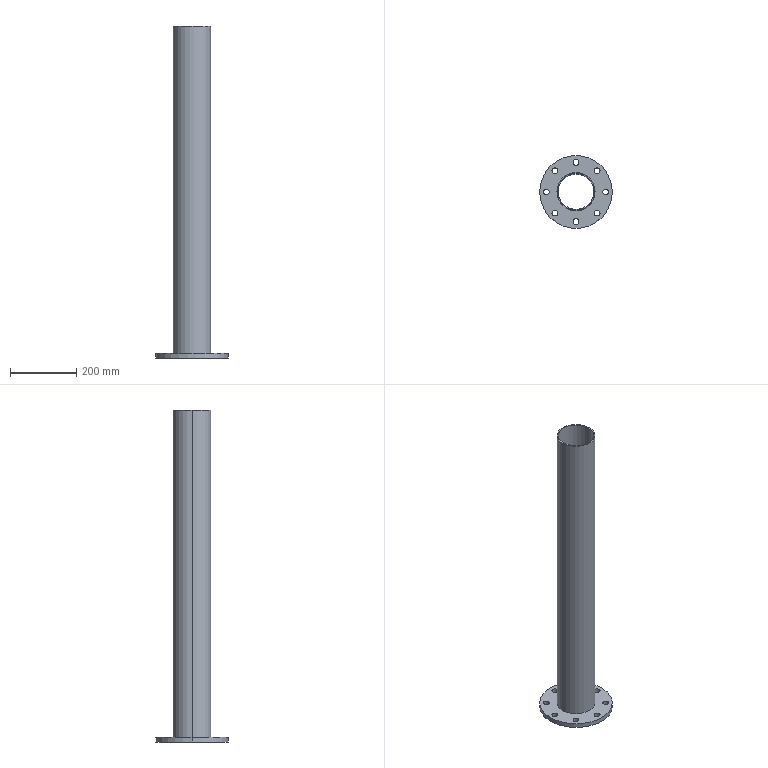Part | SolidWorks | features Extrusion 1, ICE 1 | 2 solids | 28 faces | box 220 x 220 x 1004 mm | volume 1407247 mm3 | cylinder 24 | plane 4 | commonest cylinder face diameters 18 x16 108.3 x2 114.3 x2 115 x2 220 x2
STEP:
#1=CARTESIAN_POINT('',(-72.64,63.64,14.));
#2=VERTEX_POINT('',#1);
#3=CARTESIAN_POINT('',(-54.64,63.64,14.));
#4=VERTEX_POINT('',#3);
#5=CARTESIAN_POINT('',(-63.64,63.64,14.));
#6=DIRECTION('',(0.,0.,1.));
#7=DIRECTION('',(1.,0.,0.));
#8=AXIS2_PLACEMENT_3D('',#5,#6,#7);
#9=CIRCLE('',#8,9.);
#10=EDGE_CURVE('',#2,#4,#9,.T.);
#11=ORIENTED_EDGE('',*,*,#10,.T.);
#12=CARTESIAN_POINT('',(-54.64,63.64,0.));
#13=VERTEX_POINT('',#12);
#14=CARTESIAN_POINT('',(-54.64,63.64,14.));
#15=DIRECTION('',(0.,0.,-1.));
#16=VECTOR('',#15,1000.);
#17=LINE('',#14,#16);
#18=EDGE_CURVE('',#4,#13,#17,.T.);
#19=ORIENTED_EDGE('',*,*,#18,.T.);
#20=CARTESIAN_POINT('',(-72.64,63.64,0.));
#21=VERTEX_POINT('',#20);
#22=CARTESIAN_POINT('',(-63.64,63.64,0.));
#23=DIRECTION('',(0.,0.,1.));
#24=DIRECTION('',(1.,0.,0.));
#25=AXIS2_PLACEMENT_3D('',#22,#23,#24);
#26=CIRCLE('',#25,9.);
#27=EDGE_CURVE('',#21,#13,#26,.T.);
#28=ORIENTED_EDGE('',*,*,#27,.F.);
#29=CARTESIAN_POINT('',(-72.64,63.64,14.));
#30=DIRECTION('',(0.,0.,-1.));
#31=VECTOR('',#30,1000.);
#32=LINE('',#29,#31);
#33=EDGE_CURVE('',#2,#21,#32,.T.);
#34=ORIENTED_EDGE('',*,*,#33,.F.);
#35=EDGE_LOOP('',(#11,#19,#28,#34));
#36=FACE_OUTER_BOUND('',#35,.T.);
#37=CARTESIAN_POINT('',(-63.64,63.64,14.));
#38=DIRECTION('',(0.,0.,-1.));
#39=DIRECTION('',(-1.,0.,0.));
#40=AXIS2_PLACEMENT_3D('',#37,#38,#39);
#41=CYLINDRICAL_SURFACE('',#40,9.);
#42=ADVANCED_FACE('',(#36),#41,.F.);
#43=CARTESIAN_POINT('',(-99.,0.,14.));
#44=VERTEX_POINT('',#43);
#45=CARTESIAN_POINT('',(-81.,0.,14.));
#46=VERTEX_POINT('',#45);
#47=CARTESIAN_POINT('',(-90.,0.,14.));
#48=DIRECTION('',(0.,0.,1.));
#49=DIRECTION('',(1.,0.,0.));
#50=AXIS2_PLACEMENT_3D('',#47,#48,#49);
#51=CIRCLE('',#50,9.);
#52=EDGE_CURVE('',#44,#46,#51,.T.);
#53=ORIENTED_EDGE('',*,*,#52,.T.);
#54=CARTESIAN_POINT('',(-81.,0.,0.));
#55=VERTEX_POINT('',#54);
#56=CARTESIAN_POINT('',(-81.,0.,14.));
#57=DIRECTION('',(0.,0.,-1.));
#58=VECTOR('',#57,1000.);
#59=LINE('',#56,#58);
#60=EDGE_CURVE('',#46,#55,#59,.T.);
#61=ORIENTED_EDGE('',*,*,#60,.T.);
#62=CARTESIAN_POINT('',(-99.,0.,0.));
#63=VERTEX_POINT('',#62);
#64=CARTESIAN_POINT('',(-90.,0.,0.));
#65=DIRECTION('',(0.,0.,1.));
#66=DIRECTION('',(1.,0.,0.));
#67=AXIS2_PLACEMENT_3D('',#64,#65,#66);
#68=CIRCLE('',#67,9.);
#69=EDGE_CURVE('',#63,#55,#68,.T.);
#70=ORIENTED_EDGE('',*,*,#69,.F.);
#71=CARTESIAN_POINT('',(-99.,0.,14.));
#72=DIRECTION('',(0.,0.,-1.));
#73=VECTOR('',#72,1000.);
#74=LINE('',#71,#73);
#75=EDGE_CURVE('',#44,#63,#74,.T.);
#76=ORIENTED_EDGE('',*,*,#75,.F.);
#77=EDGE_LOOP('',(#53,#61,#70,#76));
#78=FACE_OUTER_BOUND('',#77,.T.);
#79=CARTESIAN_POINT('',(-90.,0.,14.));
#80=DIRECTION('',(0.,0.,-1.));
#81=DIRECTION('',(-1.,0.,0.));
#82=AXIS2_PLACEMENT_3D('',#79,#80,#81);
#83=CYLINDRICAL_SURFACE('',#82,9.);
#84=ADVANCED_FACE('',(#78),#83,.F.);
#85=CARTESIAN_POINT('',(-72.64,-63.64,14.));
#86=VERTEX_POINT('',#85);
#87=CARTESIAN_POINT('',(-54.64,-63.64,14.));
#88=VERTEX_POINT('',#87);
#89=CARTESIAN_POINT('',(-63.64,-63.64,14.));
#90=DIRECTION('',(0.,0.,1.));
#91=DIRECTION('',(1.,0.,0.));
#92=AXIS2_PLACEMENT_3D('',#89,#90,#91);
#93=CIRCLE('',#92,9.);
#94=EDGE_CURVE('',#86,#88,#93,.T.);
#95=ORIENTED_EDGE('',*,*,#94,.T.);
#96=CARTESIAN_POINT('',(-54.64,-63.64,0.));
#97=VERTEX_POINT('',#96);
#98=CARTESIAN_POINT('',(-54.64,-63.64,14.));
#99=DIRECTION('',(0.,0.,-1.));
#100=VECTOR('',#99,1000.);
#101=LINE('',#98,#100);
#102=EDGE_CURVE('',#88,#97,#101,.T.);
#103=ORIENTED_EDGE('',*,*,#102,.T.);
#104=CARTESIAN_POINT('',(-72.64,-63.64,0.));
#105=VERTEX_POINT('',#104);
#106=CARTESIAN_POINT('',(-63.64,-63.64,0.));
#107=DIRECTION('',(0.,0.,1.));
#108=DIRECTION('',(1.,0.,0.));
#109=AXIS2_PLACEMENT_3D('',#106,#107,#108);
#110=CIRCLE('',#109,9.);
#111=EDGE_CURVE('',#105,#97,#110,.T.);
#112=ORIENTED_EDGE('',*,*,#111,.F.);
#113=CARTESIAN_POINT('',(-72.64,-63.64,14.));
#114=DIRECTION('',(0.,0.,-1.));
#115=VECTOR('',#114,1000.);
#116=LINE('',#113,#115);
#117=EDGE_CURVE('',#86,#105,#116,.T.);
#118=ORIENTED_EDGE('',*,*,#117,.F.);
#119=EDGE_LOOP('',(#95,#103,#112,#118));
#120=FACE_OUTER_BOUND('',#119,.T.);
#121=CARTESIAN_POINT('',(-63.64,-63.64,14.));
#122=DIRECTION('',(0.,0.,-1.));
#123=DIRECTION('',(-1.,0.,0.));
#124=AXIS2_PLACEMENT_3D('',#121,#122,#123);
#125=CYLINDRICAL_SURFACE('',#124,9.);
#126=ADVANCED_FACE('',(#120),#125,.F.);
#127=CARTESIAN_POINT('',(-9.,-90.,14.));
#128=VERTEX_POINT('',#127);
#129=CARTESIAN_POINT('',(9.,-90.,14.));
#130=VERTEX_POINT('',#129);
#131=CARTESIAN_POINT('',(0.,-90.,14.));
#132=DIRECTION('',(0.,0.,1.));
#133=DIRECTION('',(1.,0.,0.));
#134=AXIS2_PLACEMENT_3D('',#131,#132,#133);
#135=CIRCLE('',#134,9.);
#136=EDGE_CURVE('',#128,#130,#135,.T.);
#137=ORIENTED_EDGE('',*,*,#136,.T.);
#138=CARTESIAN_POINT('',(9.,-90.,0.));
#139=VERTEX_POINT('',#138);
#140=CARTESIAN_POINT('',(9.,-90.,14.));
#141=DIRECTION('',(0.,0.,-1.));
#142=VECTOR('',#141,1000.);
#143=LINE('',#140,#142);
#144=EDGE_CURVE('',#130,#139,#143,.T.);
#145=ORIENTED_EDGE('',*,*,#144,.T.);
#146=CARTESIAN_POINT('',(-9.,-90.,0.));
#147=VERTEX_POINT('',#146);
#148=CARTESIAN_POINT('',(0.,-90.,0.));
#149=DIRECTION('',(0.,0.,1.));
#150=DIRECTION('',(1.,0.,0.));
#151=AXIS2_PLACEMENT_3D('',#148,#149,#150);
#152=CIRCLE('',#151,9.);
#153=EDGE_CURVE('',#147,#139,#152,.T.);
#154=ORIENTED_EDGE('',*,*,#153,.F.);
#155=CARTESIAN_POINT('',(-9.,-90.,14.));
#156=DIRECTION('',(0.,0.,-1.));
#157=VECTOR('',#156,1000.);
#158=LINE('',#155,#157);
#159=EDGE_CURVE('',#128,#147,#158,.T.);
#160=ORIENTED_EDGE('',*,*,#159,.F.);
#161=EDGE_LOOP('',(#137,#145,#154,#160));
#162=FACE_OUTER_BOUND('',#161,.T.);
#163=CARTESIAN_POINT('',(0.,-90.,14.));
#164=DIRECTION('',(0.,0.,-1.));
#165=DIRECTION('',(-1.,0.,0.));
#166=AXIS2_PLACEMENT_3D('',#163,#164,#165);
#167=CYLINDRICAL_SURFACE('',#166,9.);
#168=ADVANCED_FACE('',(#162),#167,.F.);
#169=CARTESIAN_POINT('',(54.64,-63.64,14.));
#170=VERTEX_POINT('',#169);
#171=CARTESIAN_POINT('',(72.64,-63.64,14.));
#172=VERTEX_POINT('',#171);
#173=CARTESIAN_POINT('',(63.64,-63.64,14.));
#174=DIRECTION('',(0.,0.,1.));
#175=DIRECTION('',(1.,0.,0.));
#176=AXIS2_PLACEMENT_3D('',#173,#174,#175);
#177=CIRCLE('',#176,9.);
#178=EDGE_CURVE('',#170,#172,#177,.T.);
#179=ORIENTED_EDGE('',*,*,#178,.T.);
#180=CARTESIAN_POINT('',(72.64,-63.64,0.));
#181=VERTEX_POINT('',#180);
#182=CARTESIAN_POINT('',(72.64,-63.64,14.));
#183=DIRECTION('',(0.,0.,-1.));
#184=VECTOR('',#183,1000.);
#185=LINE('',#182,#184);
#186=EDGE_CURVE('',#172,#181,#185,.T.);
#187=ORIENTED_EDGE('',*,*,#186,.T.);
#188=CARTESIAN_POINT('',(54.64,-63.64,0.));
#189=VERTEX_POINT('',#188);
#190=CARTESIAN_POINT('',(63.64,-63.64,0.));
#191=DIRECTION('',(0.,0.,1.));
#192=DIRECTION('',(1.,0.,0.));
#193=AXIS2_PLACEMENT_3D('',#190,#191,#192);
#194=CIRCLE('',#193,9.);
#195=EDGE_CURVE('',#189,#181,#194,.T.);
#196=ORIENTED_EDGE('',*,*,#195,.F.);
#197=CARTESIAN_POINT('',(54.64,-63.64,14.));
#198=DIRECTION('',(0.,0.,-1.));
#199=VECTOR('',#198,1000.);
#200=LINE('',#197,#199);
#201=EDGE_CURVE('',#170,#189,#200,.T.);
#202=ORIENTED_EDGE('',*,*,#201,.F.);
#203=EDGE_LOOP('',(#179,#187,#196,#202));
#204=FACE_OUTER_BOUND('',#203,.T.);
#205=CARTESIAN_POINT('',(63.64,-63.64,14.));
#206=DIRECTION('',(0.,0.,-1.));
#207=DIRECTION('',(-1.,0.,0.));
#208=AXIS2_PLACEMENT_3D('',#205,#206,#207);
#209=CYLINDRICAL_SURFACE('',#208,9.);
#210=ADVANCED_FACE('',(#204),#209,.F.);
#211=CARTESIAN_POINT('',(81.,0.,14.));
#212=VERTEX_POINT('',#211);
#213=CARTESIAN_POINT('',(99.,0.,14.));
#214=VERTEX_POINT('',#213);
#215=CARTESIAN_POINT('',(90.,0.,14.));
#216=DIRECTION('',(0.,0.,1.));
#217=DIRECTION('',(1.,0.,0.));
#218=AXIS2_PLACEMENT_3D('',#215,#216,#217);
#219=CIRCLE('',#218,9.);
#220=EDGE_CURVE('',#212,#214,#219,.T.);
#221=ORIENTED_EDGE('',*,*,#220,.T.);
#222=CARTESIAN_POINT('',(99.,0.,0.));
#223=VERTEX_POINT('',#222);
#224=CARTESIAN_POINT('',(99.,0.,14.));
#225=DIRECTION('',(0.,0.,-1.));
#226=VECTOR('',#225,1000.);
#227=LINE('',#224,#226);
#228=EDGE_CURVE('',#214,#223,#227,.T.);
#229=ORIENTED_EDGE('',*,*,#228,.T.);
#230=CARTESIAN_POINT('',(81.,0.,0.));
#231=VERTEX_POINT('',#230);
#232=CARTESIAN_POINT('',(90.,0.,0.));
#233=DIRECTION('',(0.,0.,1.));
#234=DIRECTION('',(1.,0.,0.));
#235=AXIS2_PLACEMENT_3D('',#232,#233,#234);
#236=CIRCLE('',#235,9.);
#237=EDGE_CURVE('',#231,#223,#236,.T.);
#238=ORIENTED_EDGE('',*,*,#237,.F.);
#239=CARTESIAN_POINT('',(81.,0.,14.));
#240=DIRECTION('',(0.,0.,-1.));
#241=VECTOR('',#240,1000.);
#242=LINE('',#239,#241);
#243=EDGE_CURVE('',#212,#231,#242,.T.);
#244=ORIENTED_EDGE('',*,*,#243,.F.);
#245=EDGE_LOOP('',(#221,#229,#238,#244));
#246=FACE_OUTER_BOUND('',#245,.T.);
#247=CARTESIAN_POINT('',(90.,0.,14.));
#248=DIRECTION('',(0.,0.,-1.));
#249=DIRECTION('',(-1.,0.,0.));
#250=AXIS2_PLACEMENT_3D('',#247,#248,#249);
#251=CYLINDRICAL_SURFACE('',#250,9.);
#252=ADVANCED_FACE('',(#246),#251,.F.);
#253=CARTESIAN_POINT('',(54.64,63.64,14.));
#254=VERTEX_POINT('',#253);
#255=CARTESIAN_POINT('',(72.64,63.64,14.));
#256=VERTEX_POINT('',#255);
#257=CARTESIAN_POINT('',(63.64,63.64,14.));
#258=DIRECTION('',(0.,0.,1.));
#259=DIRECTION('',(1.,0.,0.));
#260=AXIS2_PLACEMENT_3D('',#257,#258,#259);
#261=CIRCLE('',#260,9.);
#262=EDGE_CURVE('',#254,#256,#261,.T.);
#263=ORIENTED_EDGE('',*,*,#262,.T.);
#264=CARTESIAN_POINT('',(72.64,63.64,0.));
#265=VERTEX_POINT('',#264);
#266=CARTESIAN_POINT('',(72.64,63.64,14.));
#267=DIRECTION('',(0.,0.,-1.));
#268=VECTOR('',#267,1000.);
#269=LINE('',#266,#268);
#270=EDGE_CURVE('',#256,#265,#269,.T.);
#271=ORIENTED_EDGE('',*,*,#270,.T.);
#272=CARTESIAN_POINT('',(54.64,63.64,0.));
#273=VERTEX_POINT('',#272);
#274=CARTESIAN_POINT('',(63.64,63.64,0.));
#275=DIRECTION('',(0.,0.,1.));
#276=DIRECTION('',(1.,0.,0.));
#277=AXIS2_PLACEMENT_3D('',#274,#275,#276);
#278=CIRCLE('',#277,9.);
#279=EDGE_CURVE('',#273,#265,#278,.T.);
#280=ORIENTED_EDGE('',*,*,#279,.F.);
#281=CARTESIAN_POINT('',(54.64,63.64,14.));
#282=DIRECTION('',(0.,0.,-1.));
#283=VECTOR('',#282,1000.);
#284=LINE('',#281,#283);
#285=EDGE_CURVE('',#254,#273,#284,.T.);
#286=ORIENTED_EDGE('',*,*,#285,.F.);
#287=EDGE_LOOP('',(#263,#271,#280,#286));
#288=FACE_OUTER_BOUND('',#287,.T.);
#289=CARTESIAN_POINT('',(63.64,63.64,14.));
#290=DIRECTION('',(0.,0.,-1.));
#291=DIRECTION('',(-1.,0.,0.));
#292=AXIS2_PLACEMENT_3D('',#289,#290,#291);
#293=CYLINDRICAL_SURFACE('',#292,9.);
#294=ADVANCED_FACE('',(#288),#293,.F.);
#295=CARTESIAN_POINT('',(-9.,90.,14.));
#296=VERTEX_POINT('',#295);
#297=CARTESIAN_POINT('',(9.,90.,14.));
#298=VERTEX_POINT('',#297);
#299=CARTESIAN_POINT('',(0.,90.,14.));
#300=DIRECTION('',(0.,0.,1.));
#301=DIRECTION('',(1.,0.,0.));
#302=AXIS2_PLACEMENT_3D('',#299,#300,#301);
#303=CIRCLE('',#302,9.);
#304=EDGE_CURVE('',#296,#298,#303,.T.);
#305=ORIENTED_EDGE('',*,*,#304,.T.);
#306=CARTESIAN_POINT('',(9.,90.,0.));
#307=VERTEX_POINT('',#306);
#308=CARTESIAN_POINT('',(9.,90.,14.));
#309=DIRECTION('',(0.,0.,-1.));
#310=VECTOR('',#309,1000.);
#311=LINE('',#308,#310);
#312=EDGE_CURVE('',#298,#307,#311,.T.);
#313=ORIENTED_EDGE('',*,*,#312,.T.);
#314=CARTESIAN_POINT('',(-9.,90.,0.));
#315=VERTEX_POINT('',#314);
#316=CARTESIAN_POINT('',(0.,90.,0.));
#317=DIRECTION('',(0.,0.,1.));
#318=DIRECTION('',(1.,0.,0.));
#319=AXIS2_PLACEMENT_3D('',#316,#317,#318);
#320=CIRCLE('',#319,9.);
#321=EDGE_CURVE('',#315,#307,#320,.T.);
#322=ORIENTED_EDGE('',*,*,#321,.F.);
#323=CARTESIAN_POINT('',(-9.,90.,14.));
#324=DIRECTION('',(0.,0.,-1.));
#325=VECTOR('',#324,1000.);
#326=LINE('',#323,#325);
#327=EDGE_CURVE('',#296,#315,#326,.T.);
#328=ORIENTED_EDGE('',*,*,#327,.F.);
#329=EDGE_LOOP('',(#305,#313,#322,#328));
#330=FACE_OUTER_BOUND('',#329,.T.);
#331=CARTESIAN_POINT('',(0.,90.,14.));
#332=DIRECTION('',(0.,0.,-1.));
#333=DIRECTION('',(-1.,0.,0.));
#334=AXIS2_PLACEMENT_3D('',#331,#332,#333);
#335=CYLINDRICAL_SURFACE('',#334,9.);
#336=ADVANCED_FACE('',(#330),#335,.F.);
#337=CARTESIAN_POINT('',(-57.5,0.,14.));
#338=VERTEX_POINT('',#337);
#339=CARTESIAN_POINT('',(57.5,0.,14.));
#340=VERTEX_POINT('',#339);
#341=CARTESIAN_POINT('',(0.,0.,14.));
#342=DIRECTION('',(0.,0.,1.));
#343=DIRECTION('',(1.,0.,0.));
#344=AXIS2_PLACEMENT_3D('',#341,#342,#343);
#345=CIRCLE('',#344,57.5);
#346=EDGE_CURVE('',#338,#340,#345,.T.);
#347=ORIENTED_EDGE('',*,*,#346,.T.);
#348=CARTESIAN_POINT('',(57.5,0.,0.));
#349=VERTEX_POINT('',#348);
#350=CARTESIAN_POINT('',(57.5,0.,14.));
#351=DIRECTION('',(0.,0.,-1.));
#352=VECTOR('',#351,1000.);
#353=LINE('',#350,#352);
#354=EDGE_CURVE('',#340,#349,#353,.T.);
#355=ORIENTED_EDGE('',*,*,#354,.T.);
#356=CARTESIAN_POINT('',(-57.5,0.,0.));
#357=VERTEX_POINT('',#356);
#358=CARTESIAN_POINT('',(0.,0.,0.));
#359=DIRECTION('',(0.,0.,1.));
#360=DIRECTION('',(1.,0.,0.));
#361=AXIS2_PLACEMENT_3D('',#358,#359,#360);
#362=CIRCLE('',#361,57.5);
#363=EDGE_CURVE('',#357,#349,#362,.T.);
#364=ORIENTED_EDGE('',*,*,#363,.F.);
#365=CARTESIAN_POINT('',(-57.5,0.,14.));
#366=DIRECTION('',(0.,0.,-1.));
#367=VECTOR('',#366,1000.);
#368=LINE('',#365,#367);
#369=EDGE_CURVE('',#338,#357,#368,.T.);
#370=ORIENTED_EDGE('',*,*,#369,.F.);
#371=EDGE_LOOP('',(#347,#355,#364,#370));
#372=FACE_OUTER_BOUND('',#371,.T.);
#373=CARTESIAN_POINT('',(0.,0.,14.));
#374=DIRECTION('',(0.,0.,-1.));
#375=DIRECTION('',(-1.,0.,0.));
#376=AXIS2_PLACEMENT_3D('',#373,#374,#375);
#377=CYLINDRICAL_SURFACE('',#376,57.5);
#378=ADVANCED_FACE('',(#372),#377,.F.);
#379=CARTESIAN_POINT('',(110.,0.,14.));
#380=VERTEX_POINT('',#379);
#381=CARTESIAN_POINT('',(-110.,0.,14.));
#382=VERTEX_POINT('',#381);
#383=CARTESIAN_POINT('',(0.,0.,14.));
#384=DIRECTION('',(0.,0.,1.));
#385=DIRECTION('',(1.,0.,0.));
#386=AXIS2_PLACEMENT_3D('',#383,#384,#385);
#387=CIRCLE('',#386,110.);
#388=EDGE_CURVE('',#380,#382,#387,.T.);
#389=ORIENTED_EDGE('',*,*,#388,.F.);
#390=CARTESIAN_POINT('',(110.,0.,0.));
#391=VERTEX_POINT('',#390);
#392=CARTESIAN_POINT('',(110.,0.,14.));
#393=DIRECTION('',(0.,0.,-1.));
#394=VECTOR('',#393,1000.);
#395=LINE('',#392,#394);
#396=EDGE_CURVE('',#380,#391,#395,.T.);
#397=ORIENTED_EDGE('',*,*,#396,.T.);
#398=CARTESIAN_POINT('',(-110.,0.,0.));
#399=VERTEX_POINT('',#398);
#400=CARTESIAN_POINT('',(0.,0.,0.));
#401=DIRECTION('',(0.,0.,1.));
#402=DIRECTION('',(1.,0.,0.));
#403=AXIS2_PLACEMENT_3D('',#400,#401,#402);
#404=CIRCLE('',#403,110.);
#405=EDGE_CURVE('',#391,#399,#404,.T.);
#406=ORIENTED_EDGE('',*,*,#405,.T.);
#407=CARTESIAN_POINT('',(-110.,0.,14.));
#408=DIRECTION('',(0.,0.,-1.));
#409=VECTOR('',#408,1000.);
#410=LINE('',#407,#409);
#411=EDGE_CURVE('',#382,#399,#410,.T.);
#412=ORIENTED_EDGE('',*,*,#411,.F.);
#413=EDGE_LOOP('',(#389,#397,#406,#412));
#414=FACE_OUTER_BOUND('',#413,.T.);
#415=CARTESIAN_POINT('',(0.,0.,14.));
#416=DIRECTION('',(0.,0.,-1.));
#417=DIRECTION('',(-1.,0.,0.));
#418=AXIS2_PLACEMENT_3D('',#415,#416,#417);
#419=CYLINDRICAL_SURFACE('',#418,110.);
#420=ADVANCED_FACE('',(#414),#419,.T.);
#421=ORIENTED_EDGE('',*,*,#52,.F.);
#422=CARTESIAN_POINT('',(-90.,0.,14.));
#423=DIRECTION('',(0.,0.,1.));
#424=DIRECTION('',(1.,0.,0.));
#425=AXIS2_PLACEMENT_3D('',#422,#423,#424);
#426=CIRCLE('',#425,9.);
#427=EDGE_CURVE('',#46,#44,#426,.T.);
#428=ORIENTED_EDGE('',*,*,#427,.F.);
#429=EDGE_LOOP('',(#421,#428));
#430=FACE_BOUND('',#429,.T.);
#431=ORIENTED_EDGE('',*,*,#136,.F.);
#432=CARTESIAN_POINT('',(0.,-90.,14.));
#433=DIRECTION('',(0.,0.,1.));
#434=DIRECTION('',(1.,0.,0.));
#435=AXIS2_PLACEMENT_3D('',#432,#433,#434);
#436=CIRCLE('',#435,9.);
#437=EDGE_CURVE('',#130,#128,#436,.T.);
#438=ORIENTED_EDGE('',*,*,#437,.F.);
#439=EDGE_LOOP('',(#431,#438));
#440=FACE_BOUND('',#439,.T.);
#441=ORIENTED_EDGE('',*,*,#220,.F.);
#442=CARTESIAN_POINT('',(90.,0.,14.));
#443=DIRECTION('',(0.,0.,1.));
#444=DIRECTION('',(1.,0.,0.));
#445=AXIS2_PLACEMENT_3D('',#442,#443,#444);
#446=CIRCLE('',#445,9.);
#447=EDGE_CURVE('',#214,#212,#446,.T.);
#448=ORIENTED_EDGE('',*,*,#447,.F.);
#449=EDGE_LOOP('',(#441,#448));
#450=FACE_BOUND('',#449,.T.);
#451=ORIENTED_EDGE('',*,*,#304,.F.);
#452=CARTESIAN_POINT('',(0.,90.,14.));
#453=DIRECTION('',(0.,0.,1.));
#454=DIRECTION('',(1.,0.,0.));
#455=AXIS2_PLACEMENT_3D('',#452,#453,#454);
#456=CIRCLE('',#455,9.);
#457=EDGE_CURVE('',#298,#296,#456,.T.);
#458=ORIENTED_EDGE('',*,*,#457,.F.);
#459=EDGE_LOOP('',(#451,#458));
#460=FACE_BOUND('',#459,.T.);
#461=CARTESIAN_POINT('',(0.,0.,14.));
#462=DIRECTION('',(0.,0.,1.));
#463=DIRECTION('',(1.,0.,0.));
#464=AXIS2_PLACEMENT_3D('',#461,#462,#463);
#465=CIRCLE('',#464,110.);
#466=EDGE_CURVE('',#382,#380,#465,.T.);
#467=ORIENTED_EDGE('',*,*,#466,.T.);
#468=ORIENTED_EDGE('',*,*,#388,.T.);
#469=EDGE_LOOP('',(#467,#468));
#470=FACE_OUTER_BOUND('',#469,.T.);
#471=ORIENTED_EDGE('',*,*,#346,.F.);
#472=CARTESIAN_POINT('',(0.,0.,14.));
#473=DIRECTION('',(0.,0.,1.));
#474=DIRECTION('',(1.,0.,0.));
#475=AXIS2_PLACEMENT_3D('',#472,#473,#474);
#476=CIRCLE('',#475,57.5);
#477=EDGE_CURVE('',#340,#338,#476,.T.);
#478=ORIENTED_EDGE('',*,*,#477,.F.);
#479=EDGE_LOOP('',(#471,#478));
#480=FACE_BOUND('',#479,.T.);
#481=ORIENTED_EDGE('',*,*,#262,.F.);
#482=CARTESIAN_POINT('',(63.64,63.64,14.));
#483=DIRECTION('',(0.,0.,1.));
#484=DIRECTION('',(1.,0.,0.));
#485=AXIS2_PLACEMENT_3D('',#482,#483,#484);
#486=CIRCLE('',#485,9.);
#487=EDGE_CURVE('',#256,#254,#486,.T.);
#488=ORIENTED_EDGE('',*,*,#487,.F.);
#489=EDGE_LOOP('',(#481,#488));
#490=FACE_BOUND('',#489,.T.);
#491=ORIENTED_EDGE('',*,*,#178,.F.);
#492=CARTESIAN_POINT('',(63.64,-63.64,14.));
#493=DIRECTION('',(0.,0.,1.));
#494=DIRECTION('',(1.,0.,0.));
#495=AXIS2_PLACEMENT_3D('',#492,#493,#494);
#496=CIRCLE('',#495,9.);
#497=EDGE_CURVE('',#172,#170,#496,.T.);
#498=ORIENTED_EDGE('',*,*,#497,.F.);
#499=EDGE_LOOP('',(#491,#498));
#500=FACE_BOUND('',#499,.T.);
#501=ORIENTED_EDGE('',*,*,#94,.F.);
#502=CARTESIAN_POINT('',(-63.64,-63.64,14.));
#503=DIRECTION('',(0.,0.,1.));
#504=DIRECTION('',(1.,0.,0.));
#505=AXIS2_PLACEMENT_3D('',#502,#503,#504);
#506=CIRCLE('',#505,9.);
#507=EDGE_CURVE('',#88,#86,#506,.T.);
#508=ORIENTED_EDGE('',*,*,#507,.F.);
#509=EDGE_LOOP('',(#501,#508));
#510=FACE_BOUND('',#509,.T.);
#511=ORIENTED_EDGE('',*,*,#10,.F.);
#512=CARTESIAN_POINT('',(-63.64,63.64,14.));
#513=DIRECTION('',(0.,0.,1.));
#514=DIRECTION('',(1.,0.,0.));
#515=AXIS2_PLACEMENT_3D('',#512,#513,#514);
#516=CIRCLE('',#515,9.);
#517=EDGE_CURVE('',#4,#2,#516,.T.);
#518=ORIENTED_EDGE('',*,*,#517,.F.);
#519=EDGE_LOOP('',(#511,#518));
#520=FACE_BOUND('',#519,.T.);
#521=CARTESIAN_POINT('',(0.,0.,14.));
#522=DIRECTION('',(0.,0.,1.));
#523=DIRECTION('',(1.,0.,0.));
#524=AXIS2_PLACEMENT_3D('',#521,#522,#523);
#525=PLANE('',#524);
#526=ADVANCED_FACE('',(#430,#440,#450,#460,#470,#480,#490,#500,#510,#520),#525,.T.);
#527=CARTESIAN_POINT('',(0.,0.,0.));
#528=DIRECTION('',(0.,0.,1.));
#529=DIRECTION('',(1.,0.,0.));
#530=AXIS2_PLACEMENT_3D('',#527,#528,#529);
#531=CIRCLE('',#530,110.);
#532=EDGE_CURVE('',#399,#391,#531,.T.);
#533=ORIENTED_EDGE('',*,*,#532,.F.);
#534=ORIENTED_EDGE('',*,*,#405,.F.);
#535=EDGE_LOOP('',(#533,#534));
#536=FACE_OUTER_BOUND('',#535,.T.);
#537=ORIENTED_EDGE('',*,*,#363,.T.);
#538=CARTESIAN_POINT('',(0.,0.,0.));
#539=DIRECTION('',(0.,0.,1.));
#540=DIRECTION('',(1.,0.,0.));
#541=AXIS2_PLACEMENT_3D('',#538,#539,#540);
#542=CIRCLE('',#541,57.5);
#543=EDGE_CURVE('',#349,#357,#542,.T.);
#544=ORIENTED_EDGE('',*,*,#543,.T.);
#545=EDGE_LOOP('',(#537,#544));
#546=FACE_BOUND('',#545,.T.);
#547=ORIENTED_EDGE('',*,*,#321,.T.);
#548=CARTESIAN_POINT('',(0.,90.,0.));
#549=DIRECTION('',(0.,0.,1.));
#550=DIRECTION('',(1.,0.,0.));
#551=AXIS2_PLACEMENT_3D('',#548,#549,#550);
#552=CIRCLE('',#551,9.);
#553=EDGE_CURVE('',#307,#315,#552,.T.);
#554=ORIENTED_EDGE('',*,*,#553,.T.);
#555=EDGE_LOOP('',(#547,#554));
#556=FACE_BOUND('',#555,.T.);
#557=ORIENTED_EDGE('',*,*,#279,.T.);
#558=CARTESIAN_POINT('',(63.64,63.64,0.));
#559=DIRECTION('',(0.,0.,1.));
#560=DIRECTION('',(1.,0.,0.));
#561=AXIS2_PLACEMENT_3D('',#558,#559,#560);
#562=CIRCLE('',#561,9.);
#563=EDGE_CURVE('',#265,#273,#562,.T.);
#564=ORIENTED_EDGE('',*,*,#563,.T.);
#565=EDGE_LOOP('',(#557,#564));
#566=FACE_BOUND('',#565,.T.);
#567=ORIENTED_EDGE('',*,*,#237,.T.);
#568=CARTESIAN_POINT('',(90.,0.,0.));
#569=DIRECTION('',(0.,0.,1.));
#570=DIRECTION('',(1.,0.,0.));
#571=AXIS2_PLACEMENT_3D('',#568,#569,#570);
#572=CIRCLE('',#571,9.);
#573=EDGE_CURVE('',#223,#231,#572,.T.);
#574=ORIENTED_EDGE('',*,*,#573,.T.);
#575=EDGE_LOOP('',(#567,#574));
#576=FACE_BOUND('',#575,.T.);
#577=ORIENTED_EDGE('',*,*,#195,.T.);
#578=CARTESIAN_POINT('',(63.64,-63.64,0.));
#579=DIRECTION('',(0.,0.,1.));
#580=DIRECTION('',(1.,0.,0.));
#581=AXIS2_PLACEMENT_3D('',#578,#579,#580);
#582=CIRCLE('',#581,9.);
#583=EDGE_CURVE('',#181,#189,#582,.T.);
#584=ORIENTED_EDGE('',*,*,#583,.T.);
#585=EDGE_LOOP('',(#577,#584));
#586=FACE_BOUND('',#585,.T.);
#587=ORIENTED_EDGE('',*,*,#153,.T.);
#588=CARTESIAN_POINT('',(0.,-90.,0.));
#589=DIRECTION('',(0.,0.,1.));
#590=DIRECTION('',(1.,0.,0.));
#591=AXIS2_PLACEMENT_3D('',#588,#589,#590);
#592=CIRCLE('',#591,9.);
#593=EDGE_CURVE('',#139,#147,#592,.T.);
#594=ORIENTED_EDGE('',*,*,#593,.T.);
#595=EDGE_LOOP('',(#587,#594));
#596=FACE_BOUND('',#595,.T.);
#597=ORIENTED_EDGE('',*,*,#111,.T.);
#598=CARTESIAN_POINT('',(-63.64,-63.64,0.));
#599=DIRECTION('',(0.,0.,1.));
#600=DIRECTION('',(1.,0.,0.));
#601=AXIS2_PLACEMENT_3D('',#598,#599,#600);
#602=CIRCLE('',#601,9.);
#603=EDGE_CURVE('',#97,#105,#602,.T.);
#604=ORIENTED_EDGE('',*,*,#603,.T.);
#605=EDGE_LOOP('',(#597,#604));
#606=FACE_BOUND('',#605,.T.);
#607=ORIENTED_EDGE('',*,*,#69,.T.);
#608=CARTESIAN_POINT('',(-90.,0.,0.));
#609=DIRECTION('',(0.,0.,1.));
#610=DIRECTION('',(1.,0.,0.));
#611=AXIS2_PLACEMENT_3D('',#608,#609,#610);
#612=CIRCLE('',#611,9.);
#613=EDGE_CURVE('',#55,#63,#612,.T.);
#614=ORIENTED_EDGE('',*,*,#613,.T.);
#615=EDGE_LOOP('',(#607,#614));
#616=FACE_BOUND('',#615,.T.);
#617=ORIENTED_EDGE('',*,*,#27,.T.);
#618=CARTESIAN_POINT('',(-63.64,63.64,0.));
#619=DIRECTION('',(0.,0.,1.));
#620=DIRECTION('',(1.,0.,0.));
#621=AXIS2_PLACEMENT_3D('',#618,#619,#620);
#622=CIRCLE('',#621,9.);
#623=EDGE_CURVE('',#13,#21,#622,.T.);
#624=ORIENTED_EDGE('',*,*,#623,.T.);
#625=EDGE_LOOP('',(#617,#624));
#626=FACE_BOUND('',#625,.T.);
#627=CARTESIAN_POINT('',(0.,0.,0.));
#628=DIRECTION('',(0.,0.,1.));
#629=DIRECTION('',(1.,0.,0.));
#630=AXIS2_PLACEMENT_3D('',#627,#628,#629);
#631=PLANE('',#630);
#632=ADVANCED_FACE('',(#536,#546,#556,#566,#576,#586,#596,#606,#616,#626),#631,.F.);
#633=ORIENTED_EDGE('',*,*,#396,.F.);
#634=ORIENTED_EDGE('',*,*,#466,.F.);
#635=ORIENTED_EDGE('',*,*,#411,.T.);
#636=ORIENTED_EDGE('',*,*,#532,.T.);
#637=EDGE_LOOP('',(#633,#634,#635,#636));
#638=FACE_OUTER_BOUND('',#637,.T.);
#639=CARTESIAN_POINT('',(0.,0.,14.));
#640=DIRECTION('',(0.,0.,-1.));
#641=DIRECTION('',(-1.,0.,0.));
#642=AXIS2_PLACEMENT_3D('',#639,#640,#641);
#643=CYLINDRICAL_SURFACE('',#642,110.);
#644=ADVANCED_FACE('',(#638),#643,.T.);
#645=ORIENTED_EDGE('',*,*,#354,.F.);
#646=ORIENTED_EDGE('',*,*,#477,.T.);
#647=ORIENTED_EDGE('',*,*,#369,.T.);
#648=ORIENTED_EDGE('',*,*,#543,.F.);
#649=EDGE_LOOP('',(#645,#646,#647,#648));
#650=FACE_OUTER_BOUND('',#649,.T.);
#651=CARTESIAN_POINT('',(0.,0.,14.));
#652=DIRECTION('',(0.,0.,-1.));
#653=DIRECTION('',(-1.,0.,0.));
#654=AXIS2_PLACEMENT_3D('',#651,#652,#653);
#655=CYLINDRICAL_SURFACE('',#654,57.5);
#656=ADVANCED_FACE('',(#650),#655,.F.);
#657=ORIENTED_EDGE('',*,*,#312,.F.);
#658=ORIENTED_EDGE('',*,*,#457,.T.);
#659=ORIENTED_EDGE('',*,*,#327,.T.);
#660=ORIENTED_EDGE('',*,*,#553,.F.);
#661=EDGE_LOOP('',(#657,#658,#659,#660));
#662=FACE_OUTER_BOUND('',#661,.T.);
#663=CARTESIAN_POINT('',(0.,90.,14.));
#664=DIRECTION('',(0.,0.,-1.));
#665=DIRECTION('',(-1.,0.,0.));
#666=AXIS2_PLACEMENT_3D('',#663,#664,#665);
#667=CYLINDRICAL_SURFACE('',#666,9.);
#668=ADVANCED_FACE('',(#662),#667,.F.);
#669=ORIENTED_EDGE('',*,*,#270,.F.);
#670=ORIENTED_EDGE('',*,*,#487,.T.);
#671=ORIENTED_EDGE('',*,*,#285,.T.);
#672=ORIENTED_EDGE('',*,*,#563,.F.);
#673=EDGE_LOOP('',(#669,#670,#671,#672));
#674=FACE_OUTER_BOUND('',#673,.T.);
#675=CARTESIAN_POINT('',(63.64,63.64,14.));
#676=DIRECTION('',(0.,0.,-1.));
#677=DIRECTION('',(-1.,0.,0.));
#678=AXIS2_PLACEMENT_3D('',#675,#676,#677);
#679=CYLINDRICAL_SURFACE('',#678,9.);
#680=ADVANCED_FACE('',(#674),#679,.F.);
#681=ORIENTED_EDGE('',*,*,#228,.F.);
#682=ORIENTED_EDGE('',*,*,#447,.T.);
#683=ORIENTED_EDGE('',*,*,#243,.T.);
#684=ORIENTED_EDGE('',*,*,#573,.F.);
#685=EDGE_LOOP('',(#681,#682,#683,#684));
#686=FACE_OUTER_BOUND('',#685,.T.);
#687=CARTESIAN_POINT('',(90.,0.,14.));
#688=DIRECTION('',(0.,0.,-1.));
#689=DIRECTION('',(-1.,0.,0.));
#690=AXIS2_PLACEMENT_3D('',#687,#688,#689);
#691=CYLINDRICAL_SURFACE('',#690,9.);
#692=ADVANCED_FACE('',(#686),#691,.F.);
#693=ORIENTED_EDGE('',*,*,#186,.F.);
#694=ORIENTED_EDGE('',*,*,#497,.T.);
#695=ORIENTED_EDGE('',*,*,#201,.T.);
#696=ORIENTED_EDGE('',*,*,#583,.F.);
#697=EDGE_LOOP('',(#693,#694,#695,#696));
#698=FACE_OUTER_BOUND('',#697,.T.);
#699=CARTESIAN_POINT('',(63.64,-63.64,14.));
#700=DIRECTION('',(0.,0.,-1.));
#701=DIRECTION('',(-1.,0.,0.));
#702=AXIS2_PLACEMENT_3D('',#699,#700,#701);
#703=CYLINDRICAL_SURFACE('',#702,9.);
#704=ADVANCED_FACE('',(#698),#703,.F.);
#705=ORIENTED_EDGE('',*,*,#144,.F.);
#706=ORIENTED_EDGE('',*,*,#437,.T.);
#707=ORIENTED_EDGE('',*,*,#159,.T.);
#708=ORIENTED_EDGE('',*,*,#593,.F.);
#709=EDGE_LOOP('',(#705,#706,#707,#708));
#710=FACE_OUTER_BOUND('',#709,.T.);
#711=CARTESIAN_POINT('',(0.,-90.,14.));
#712=DIRECTION('',(0.,0.,-1.));
#713=DIRECTION('',(-1.,0.,0.));
#714=AXIS2_PLACEMENT_3D('',#711,#712,#713);
#715=CYLINDRICAL_SURFACE('',#714,9.);
#716=ADVANCED_FACE('',(#710),#715,.F.);
#717=ORIENTED_EDGE('',*,*,#102,.F.);
#718=ORIENTED_EDGE('',*,*,#507,.T.);
#719=ORIENTED_EDGE('',*,*,#117,.T.);
#720=ORIENTED_EDGE('',*,*,#603,.F.);
#721=EDGE_LOOP('',(#717,#718,#719,#720));
#722=FACE_OUTER_BOUND('',#721,.T.);
#723=CARTESIAN_POINT('',(-63.64,-63.64,14.));
#724=DIRECTION('',(0.,0.,-1.));
#725=DIRECTION('',(-1.,0.,0.));
#726=AXIS2_PLACEMENT_3D('',#723,#724,#725);
#727=CYLINDRICAL_SURFACE('',#726,9.);
#728=ADVANCED_FACE('',(#722),#727,.F.);
#729=ORIENTED_EDGE('',*,*,#60,.F.);
#730=ORIENTED_EDGE('',*,*,#427,.T.);
#731=ORIENTED_EDGE('',*,*,#75,.T.);
#732=ORIENTED_EDGE('',*,*,#613,.F.);
#733=EDGE_LOOP('',(#729,#730,#731,#732));
#734=FACE_OUTER_BOUND('',#733,.T.);
#735=CARTESIAN_POINT('',(-90.,0.,14.));
#736=DIRECTION('',(0.,0.,-1.));
#737=DIRECTION('',(-1.,0.,0.));
#738=AXIS2_PLACEMENT_3D('',#735,#736,#737);
#739=CYLINDRICAL_SURFACE('',#738,9.);
#740=ADVANCED_FACE('',(#734),#739,.F.);
#741=ORIENTED_EDGE('',*,*,#18,.F.);
#742=ORIENTED_EDGE('',*,*,#517,.T.);
#743=ORIENTED_EDGE('',*,*,#33,.T.);
#744=ORIENTED_EDGE('',*,*,#623,.F.);
#745=EDGE_LOOP('',(#741,#742,#743,#744));
#746=FACE_OUTER_BOUND('',#745,.T.);
#747=CARTESIAN_POINT('',(-63.64,63.64,14.));
#748=DIRECTION('',(0.,0.,-1.));
#749=DIRECTION('',(-1.,0.,0.));
#750=AXIS2_PLACEMENT_3D('',#747,#748,#749);
#751=CYLINDRICAL_SURFACE('',#750,9.);
#752=ADVANCED_FACE('',(#746),#751,.F.);
#753=CLOSED_SHELL('',(#42,#84,#126,#168,#210,#252,#294,#336,#378,#420,#526,#632,#644,#656,#668,#680,#692,#704,#716,#728,#740,#752));
#754=MANIFOLD_SOLID_BREP('',#753);
#755=CARTESIAN_POINT('',(-54.15,0.,1004.));
#756=VERTEX_POINT('',#755);
#757=CARTESIAN_POINT('',(54.15,0.,1004.));
#758=VERTEX_POINT('',#757);
#759=CARTESIAN_POINT('',(0.,0.,1004.));
#760=DIRECTION('',(0.,0.,1.));
#761=DIRECTION('',(1.,0.,0.));
#762=AXIS2_PLACEMENT_3D('',#759,#760,#761);
#763=CIRCLE('',#762,54.15);
#764=EDGE_CURVE('',#756,#758,#763,.T.);
#765=ORIENTED_EDGE('',*,*,#764,.T.);
#766=CARTESIAN_POINT('',(54.15,0.,4.));
#767=VERTEX_POINT('',#766);
#768=CARTESIAN_POINT('',(54.15,0.,1004.));
#769=DIRECTION('',(0.,0.,-1.));
#770=VECTOR('',#769,1000.);
#771=LINE('',#768,#770);
#772=EDGE_CURVE('',#758,#767,#771,.T.);
#773=ORIENTED_EDGE('',*,*,#772,.T.);
#774=CARTESIAN_POINT('',(-54.15,0.,4.));
#775=VERTEX_POINT('',#774);
#776=CARTESIAN_POINT('',(0.,0.,4.));
#777=DIRECTION('',(0.,0.,1.));
#778=DIRECTION('',(1.,0.,0.));
#779=AXIS2_PLACEMENT_3D('',#776,#777,#778);
#780=CIRCLE('',#779,54.15);
#781=EDGE_CURVE('',#775,#767,#780,.T.);
#782=ORIENTED_EDGE('',*,*,#781,.F.);
#783=CARTESIAN_POINT('',(-54.15,0.,1004.));
#784=DIRECTION('',(0.,0.,-1.));
#785=VECTOR('',#784,1000.);
#786=LINE('',#783,#785);
#787=EDGE_CURVE('',#756,#775,#786,.T.);
#788=ORIENTED_EDGE('',*,*,#787,.F.);
#789=EDGE_LOOP('',(#765,#773,#782,#788));
#790=FACE_OUTER_BOUND('',#789,.T.);
#791=CARTESIAN_POINT('',(0.,0.,1004.));
#792=DIRECTION('',(0.,0.,-1.));
#793=DIRECTION('',(-1.,0.,0.));
#794=AXIS2_PLACEMENT_3D('',#791,#792,#793);
#795=CYLINDRICAL_SURFACE('',#794,54.15);
#796=ADVANCED_FACE('',(#790),#795,.F.);
#797=CARTESIAN_POINT('',(57.15,0.,1004.));
#798=VERTEX_POINT('',#797);
#799=CARTESIAN_POINT('',(-57.15,0.,1004.));
#800=VERTEX_POINT('',#799);
#801=CARTESIAN_POINT('',(0.,0.,1004.));
#802=DIRECTION('',(0.,0.,1.));
#803=DIRECTION('',(1.,0.,0.));
#804=AXIS2_PLACEMENT_3D('',#801,#802,#803);
#805=CIRCLE('',#804,57.15);
#806=EDGE_CURVE('',#798,#800,#805,.T.);
#807=ORIENTED_EDGE('',*,*,#806,.F.);
#808=CARTESIAN_POINT('',(57.15,0.,4.));
#809=VERTEX_POINT('',#808);
#810=CARTESIAN_POINT('',(57.15,0.,1004.));
#811=DIRECTION('',(0.,0.,-1.));
#812=VECTOR('',#811,1000.);
#813=LINE('',#810,#812);
#814=EDGE_CURVE('',#798,#809,#813,.T.);
#815=ORIENTED_EDGE('',*,*,#814,.T.);
#816=CARTESIAN_POINT('',(-57.15,0.,4.));
#817=VERTEX_POINT('',#816);
#818=CARTESIAN_POINT('',(0.,0.,4.));
#819=DIRECTION('',(0.,0.,1.));
#820=DIRECTION('',(1.,0.,0.));
#821=AXIS2_PLACEMENT_3D('',#818,#819,#820);
#822=CIRCLE('',#821,57.15);
#823=EDGE_CURVE('',#809,#817,#822,.T.);
#824=ORIENTED_EDGE('',*,*,#823,.T.);
#825=CARTESIAN_POINT('',(-57.15,0.,1004.));
#826=DIRECTION('',(0.,0.,-1.));
#827=VECTOR('',#826,1000.);
#828=LINE('',#825,#827);
#829=EDGE_CURVE('',#800,#817,#828,.T.);
#830=ORIENTED_EDGE('',*,*,#829,.F.);
#831=EDGE_LOOP('',(#807,#815,#824,#830));
#832=FACE_OUTER_BOUND('',#831,.T.);
#833=CARTESIAN_POINT('',(0.,0.,1004.));
#834=DIRECTION('',(0.,0.,-1.));
#835=DIRECTION('',(-1.,0.,0.));
#836=AXIS2_PLACEMENT_3D('',#833,#834,#835);
#837=CYLINDRICAL_SURFACE('',#836,57.15);
#838=ADVANCED_FACE('',(#832),#837,.T.);
#839=CARTESIAN_POINT('',(0.,0.,1004.));
#840=DIRECTION('',(0.,0.,1.));
#841=DIRECTION('',(1.,0.,0.));
#842=AXIS2_PLACEMENT_3D('',#839,#840,#841);
#843=CIRCLE('',#842,57.15);
#844=EDGE_CURVE('',#800,#798,#843,.T.);
#845=ORIENTED_EDGE('',*,*,#844,.T.);
#846=ORIENTED_EDGE('',*,*,#806,.T.);
#847=EDGE_LOOP('',(#845,#846));
#848=FACE_OUTER_BOUND('',#847,.T.);
#849=ORIENTED_EDGE('',*,*,#764,.F.);
#850=CARTESIAN_POINT('',(0.,0.,1004.));
#851=DIRECTION('',(0.,0.,1.));
#852=DIRECTION('',(1.,0.,0.));
#853=AXIS2_PLACEMENT_3D('',#850,#851,#852);
#854=CIRCLE('',#853,54.15);
#855=EDGE_CURVE('',#758,#756,#854,.T.);
#856=ORIENTED_EDGE('',*,*,#855,.F.);
#857=EDGE_LOOP('',(#849,#856));
#858=FACE_BOUND('',#857,.T.);
#859=CARTESIAN_POINT('',(0.,0.,1004.));
#860=DIRECTION('',(0.,0.,1.));
#861=DIRECTION('',(1.,0.,0.));
#862=AXIS2_PLACEMENT_3D('',#859,#860,#861);
#863=PLANE('',#862);
#864=ADVANCED_FACE('',(#848,#858),#863,.T.);
#865=CARTESIAN_POINT('',(0.,0.,4.));
#866=DIRECTION('',(0.,0.,1.));
#867=DIRECTION('',(1.,0.,0.));
#868=AXIS2_PLACEMENT_3D('',#865,#866,#867);
#869=CIRCLE('',#868,57.15);
#870=EDGE_CURVE('',#817,#809,#869,.T.);
#871=ORIENTED_EDGE('',*,*,#870,.F.);
#872=ORIENTED_EDGE('',*,*,#823,.F.);
#873=EDGE_LOOP('',(#871,#872));
#874=FACE_OUTER_BOUND('',#873,.T.);
#875=ORIENTED_EDGE('',*,*,#781,.T.);
#876=CARTESIAN_POINT('',(0.,0.,4.));
#877=DIRECTION('',(0.,0.,1.));
#878=DIRECTION('',(1.,0.,0.));
#879=AXIS2_PLACEMENT_3D('',#876,#877,#878);
#880=CIRCLE('',#879,54.15);
#881=EDGE_CURVE('',#767,#775,#880,.T.);
#882=ORIENTED_EDGE('',*,*,#881,.T.);
#883=EDGE_LOOP('',(#875,#882));
#884=FACE_BOUND('',#883,.T.);
#885=CARTESIAN_POINT('',(0.,0.,4.));
#886=DIRECTION('',(0.,0.,1.));
#887=DIRECTION('',(1.,0.,0.));
#888=AXIS2_PLACEMENT_3D('',#885,#886,#887);
#889=PLANE('',#888);
#890=ADVANCED_FACE('',(#874,#884),#889,.F.);
#891=ORIENTED_EDGE('',*,*,#814,.F.);
#892=ORIENTED_EDGE('',*,*,#844,.F.);
#893=ORIENTED_EDGE('',*,*,#829,.T.);
#894=ORIENTED_EDGE('',*,*,#870,.T.);
#895=EDGE_LOOP('',(#891,#892,#893,#894));
#896=FACE_OUTER_BOUND('',#895,.T.);
#897=CARTESIAN_POINT('',(0.,0.,1004.));
#898=DIRECTION('',(0.,0.,-1.));
#899=DIRECTION('',(-1.,0.,0.));
#900=AXIS2_PLACEMENT_3D('',#897,#898,#899);
#901=CYLINDRICAL_SURFACE('',#900,57.15);
#902=ADVANCED_FACE('',(#896),#901,.T.);
#903=ORIENTED_EDGE('',*,*,#772,.F.);
#904=ORIENTED_EDGE('',*,*,#855,.T.);
#905=ORIENTED_EDGE('',*,*,#787,.T.);
#906=ORIENTED_EDGE('',*,*,#881,.F.);
#907=EDGE_LOOP('',(#903,#904,#905,#906));
#908=FACE_OUTER_BOUND('',#907,.T.);
#909=CARTESIAN_POINT('',(0.,0.,1004.));
#910=DIRECTION('',(0.,0.,-1.));
#911=DIRECTION('',(-1.,0.,0.));
#912=AXIS2_PLACEMENT_3D('',#909,#910,#911);
#913=CYLINDRICAL_SURFACE('',#912,54.15);
#914=ADVANCED_FACE('',(#908),#913,.F.);
#915=CLOSED_SHELL('',(#796,#838,#864,#890,#902,#914));
#916=MANIFOLD_SOLID_BREP('',#915);
#917=CARTESIAN_POINT('',(0.,0.,0.));
#918=DIRECTION('',(0.,0.,1.));
#919=DIRECTION('',(1.,0.,0.));
#920=AXIS2_PLACEMENT_3D('',#917,#918,#919);
#921=(LENGTH_UNIT()NAMED_UNIT(*)SI_UNIT(.MILLI.,.METRE.));
#922=UNCERTAINTY_MEASURE_WITH_UNIT(LENGTH_MEASURE(0.00001),#921,'','');
#923=(NAMED_UNIT(*)PLANE_ANGLE_UNIT()SI_UNIT($,.RADIAN.));
#924=(NAMED_UNIT(*)SI_UNIT($,.STERADIAN.)SOLID_ANGLE_UNIT());
#925=(GEOMETRIC_REPRESENTATION_CONTEXT(3)GLOBAL_UNCERTAINTY_ASSIGNED_CONTEXT((#922))GLOBAL_UNIT_ASSIGNED_CONTEXT((#921,#923,#924))REPRESENTATION_CONTEXT('',''));
#926=ADVANCED_BREP_SHAPE_REPRESENTATION('',(#754,#916,#920),#925);